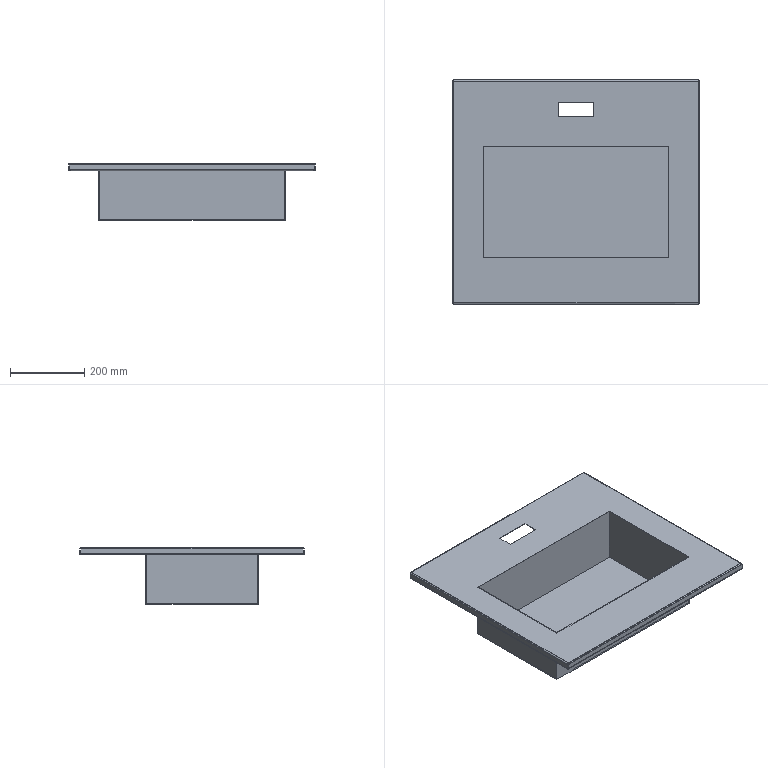Part | SolidWorks | features ICE 3, EdgeFlange 2, FlatPattern 1, SMBaseFlange 1, SheetMetal 1 | 1 solid | 84 faces | box 665 x 605 x 153.5 mm | volume 1290484 mm3 | plane 52 | spline 16 | cylinder 16 | commonest cylinder face diameters 4 x8 7 x8